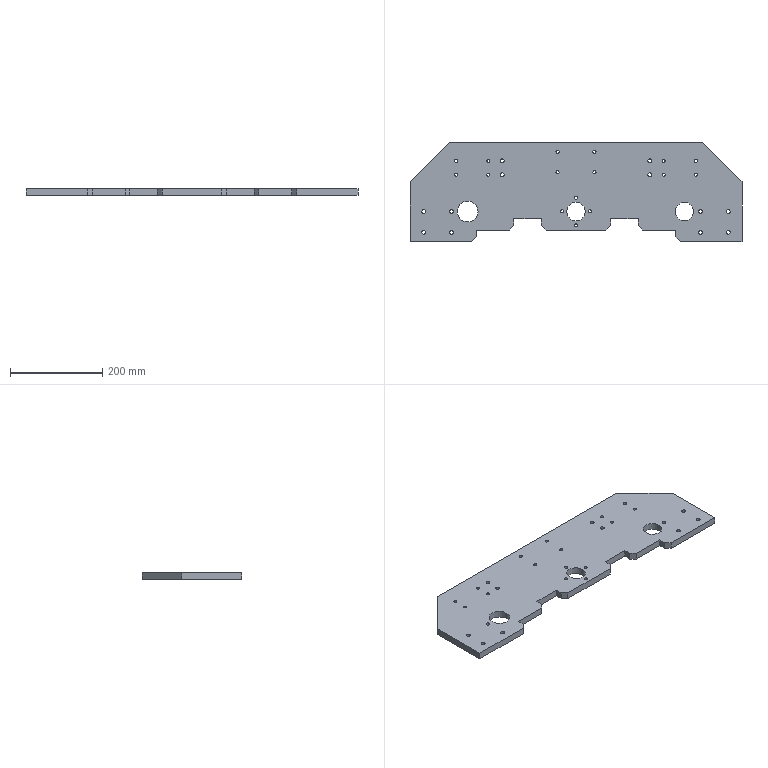Part | SolidWorks | features BaseBody 1 | 1 solid | 88 faces | box 720 x 215 x 15 mm | volume 1921061 mm3 | cylinder 62 | plane 26 | commonest cylinder face diameters 6.8 x32 8.5 x24 40 x4 45 x2